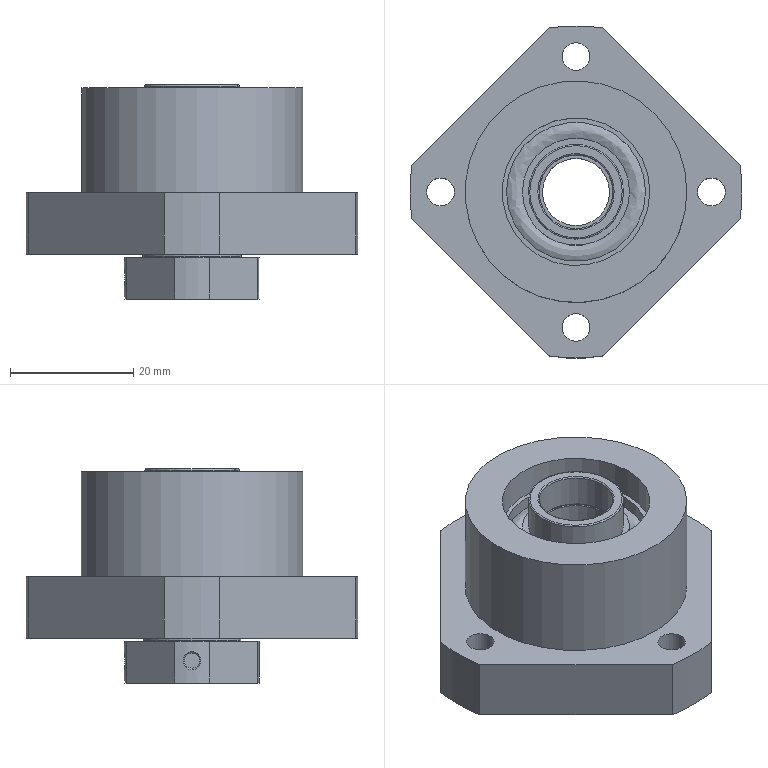Part | STEP file | 1 solid | 81 faces | box 54 x 54 x 34.8 mm | volume 31485 mm3 | cylinder 34 | plane 28 | spline 14 | cone 5 | commonest cylinder face diameters 4.5 x4 8 x4 12 x4 22 x4 54 x4 28 x3